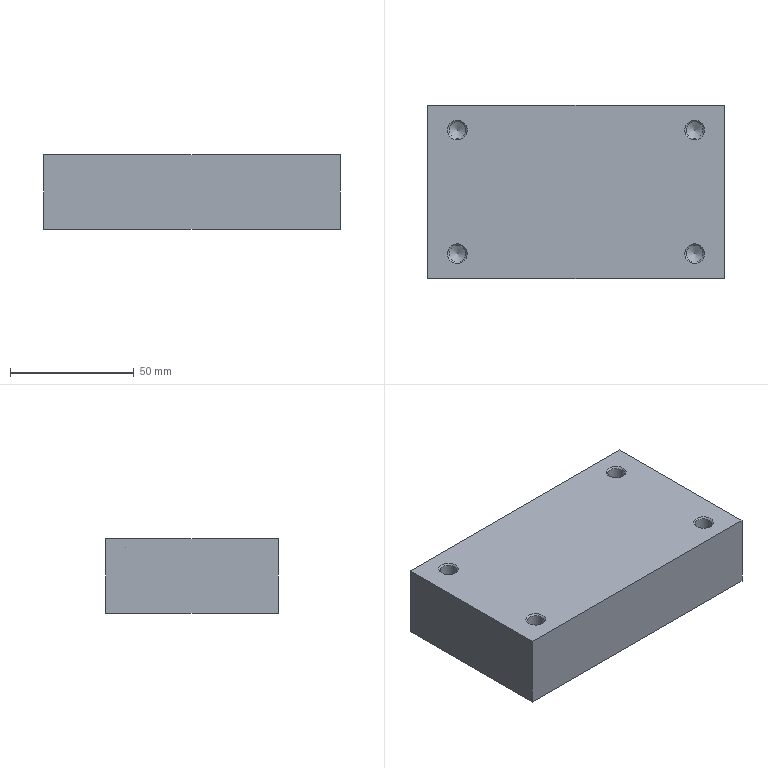Part | STEP file | 冲床-300配套压波_id858_x_t | 1 solid | 18 faces | box 120 x 70 x 30 mm | volume 248979 mm3 | cone 8 | plane 6 | cylinder 4 | commonest cylinder face diameters 6.8 x4
STEP:
#1=CARTESIAN_POINT('',(1760.4,25.,88.));
#2=VERTEX_POINT('',#1);
#3=CARTESIAN_POINT('',(1757.,25.,88.));
#4=DIRECTION('',(0.,0.,1.));
#5=DIRECTION('',(1.,0.,0.));
#6=AXIS2_PLACEMENT_3D('',#3,#4,#5);
#7=CIRCLE('',#6,3.4);
#8=EDGE_CURVE('',#2,#2,#7,.T.);
#9=ORIENTED_EDGE('',*,*,#8,.T.);
#10=EDGE_LOOP('',(#9));
#11=FACE_BOUND('',#10,.T.);
#12=CARTESIAN_POINT('',(1757.,25.,85.957));
#13=VERTEX_POINT('',#12);
#14=VERTEX_LOOP('',#13);
#15=FACE_BOUND('',#14,.T.);
#16=CARTESIAN_POINT('',(1757.,25.,88.));
#17=DIRECTION('',(0.,0.,1.));
#18=DIRECTION('',(-1.,0.,0.));
#19=AXIS2_PLACEMENT_3D('',#16,#17,#18);
#20=CONICAL_SURFACE('',#19,3.4,59.);
#21=ADVANCED_FACE('',(#11,#15),#20,.F.);
#22=CARTESIAN_POINT('',(1753.6,25.,107.4));
#23=VERTEX_POINT('',#22);
#24=CARTESIAN_POINT('',(1757.,25.,107.4));
#25=DIRECTION('',(0.,0.,1.));
#26=DIRECTION('',(-1.,0.,0.));
#27=AXIS2_PLACEMENT_3D('',#24,#25,#26);
#28=CIRCLE('',#27,3.4);
#29=EDGE_CURVE('',#23,#23,#28,.T.);
#30=ORIENTED_EDGE('',*,*,#29,.T.);
#31=EDGE_LOOP('',(#30));
#32=FACE_BOUND('',#31,.T.);
#33=ORIENTED_EDGE('',*,*,#8,.F.);
#34=EDGE_LOOP('',(#33));
#35=FACE_BOUND('',#34,.T.);
#36=CARTESIAN_POINT('',(1757.,25.,108.));
#37=DIRECTION('',(0.,0.,-1.));
#38=DIRECTION('',(1.,0.,0.));
#39=AXIS2_PLACEMENT_3D('',#36,#37,#38);
#40=CYLINDRICAL_SURFACE('',#39,3.4);
#41=ADVANCED_FACE('',(#32,#35),#40,.F.);
#42=ORIENTED_EDGE('',*,*,#29,.F.);
#43=EDGE_LOOP('',(#42));
#44=FACE_BOUND('',#43,.T.);
#45=CARTESIAN_POINT('',(1753.,25.,108.));
#46=VERTEX_POINT('',#45);
#47=CARTESIAN_POINT('',(1757.,25.,108.));
#48=DIRECTION('',(0.,0.,-1.));
#49=DIRECTION('',(-1.,0.,0.));
#50=AXIS2_PLACEMENT_3D('',#47,#48,#49);
#51=CIRCLE('',#50,4.);
#52=EDGE_CURVE('',#46,#46,#51,.T.);
#53=ORIENTED_EDGE('',*,*,#52,.F.);
#54=EDGE_LOOP('',(#53));
#55=FACE_BOUND('',#54,.T.);
#56=CARTESIAN_POINT('',(1757.,25.,108.));
#57=DIRECTION('',(0.,0.,1.));
#58=DIRECTION('',(-1.,0.,0.));
#59=AXIS2_PLACEMENT_3D('',#56,#57,#58);
#60=CONICAL_SURFACE('',#59,4.,45.);
#61=ADVANCED_FACE('',(#44,#55),#60,.F.);
#62=CARTESIAN_POINT('',(1849.6,25.,88.));
#63=VERTEX_POINT('',#62);
#64=CARTESIAN_POINT('',(1853.,25.,88.));
#65=DIRECTION('',(0.,0.,1.));
#66=DIRECTION('',(-1.,0.,0.));
#67=AXIS2_PLACEMENT_3D('',#64,#65,#66);
#68=CIRCLE('',#67,3.4);
#69=EDGE_CURVE('',#63,#63,#68,.T.);
#70=ORIENTED_EDGE('',*,*,#69,.T.);
#71=EDGE_LOOP('',(#70));
#72=FACE_BOUND('',#71,.T.);
#73=CARTESIAN_POINT('',(1853.,25.,85.957));
#74=VERTEX_POINT('',#73);
#75=VERTEX_LOOP('',#74);
#76=FACE_BOUND('',#75,.T.);
#77=CARTESIAN_POINT('',(1853.,25.,88.));
#78=DIRECTION('',(0.,0.,1.));
#79=DIRECTION('',(1.,0.,0.));
#80=AXIS2_PLACEMENT_3D('',#77,#78,#79);
#81=CONICAL_SURFACE('',#80,3.4,59.);
#82=ADVANCED_FACE('',(#72,#76),#81,.F.);
#83=CARTESIAN_POINT('',(1849.6,-25.,88.));
#84=VERTEX_POINT('',#83);
#85=CARTESIAN_POINT('',(1853.,-25.,88.));
#86=DIRECTION('',(0.,0.,1.));
#87=DIRECTION('',(-1.,0.,0.));
#88=AXIS2_PLACEMENT_3D('',#85,#86,#87);
#89=CIRCLE('',#88,3.4);
#90=EDGE_CURVE('',#84,#84,#89,.T.);
#91=ORIENTED_EDGE('',*,*,#90,.T.);
#92=EDGE_LOOP('',(#91));
#93=FACE_BOUND('',#92,.T.);
#94=CARTESIAN_POINT('',(1853.,-25.,85.957));
#95=VERTEX_POINT('',#94);
#96=VERTEX_LOOP('',#95);
#97=FACE_BOUND('',#96,.T.);
#98=CARTESIAN_POINT('',(1853.,-25.,88.));
#99=DIRECTION('',(0.,0.,1.));
#100=DIRECTION('',(1.,0.,0.));
#101=AXIS2_PLACEMENT_3D('',#98,#99,#100);
#102=CONICAL_SURFACE('',#101,3.4,59.);
#103=ADVANCED_FACE('',(#93,#97),#102,.F.);
#104=CARTESIAN_POINT('',(1745.,35.,78.));
#105=VERTEX_POINT('',#104);
#106=CARTESIAN_POINT('',(1745.,-35.,78.));
#107=VERTEX_POINT('',#106);
#108=CARTESIAN_POINT('',(1745.,0.,78.));
#109=DIRECTION('',(0.,-1.,0.));
#110=VECTOR('',#109,1.);
#111=LINE('',#108,#110);
#112=EDGE_CURVE('',#105,#107,#111,.T.);
#113=ORIENTED_EDGE('',*,*,#112,.F.);
#114=CARTESIAN_POINT('',(1865.,35.,78.));
#115=VERTEX_POINT('',#114);
#116=CARTESIAN_POINT('',(60.,35.,78.));
#117=DIRECTION('',(-1.,0.,0.));
#118=VECTOR('',#117,1.);
#119=LINE('',#116,#118);
#120=EDGE_CURVE('',#115,#105,#119,.T.);
#121=ORIENTED_EDGE('',*,*,#120,.F.);
#122=CARTESIAN_POINT('',(1865.,-35.,78.));
#123=VERTEX_POINT('',#122);
#124=CARTESIAN_POINT('',(1865.,0.,78.));
#125=DIRECTION('',(0.,1.,0.));
#126=VECTOR('',#125,1.);
#127=LINE('',#124,#126);
#128=EDGE_CURVE('',#123,#115,#127,.T.);
#129=ORIENTED_EDGE('',*,*,#128,.F.);
#130=CARTESIAN_POINT('',(60.,-35.,78.));
#131=DIRECTION('',(1.,0.,0.));
#132=VECTOR('',#131,1.);
#133=LINE('',#130,#132);
#134=EDGE_CURVE('',#107,#123,#133,.T.);
#135=ORIENTED_EDGE('',*,*,#134,.F.);
#136=EDGE_LOOP('',(#113,#121,#129,#135));
#137=FACE_OUTER_BOUND('',#136,.T.);
#138=CARTESIAN_POINT('',(60.,0.,78.));
#139=DIRECTION('',(0.,0.,1.));
#140=DIRECTION('',(1.,0.,0.));
#141=AXIS2_PLACEMENT_3D('',#138,#139,#140);
#142=PLANE('',#141);
#143=ADVANCED_FACE('',(#137),#142,.F.);
#144=CARTESIAN_POINT('',(1856.4,25.,107.4));
#145=VERTEX_POINT('',#144);
#146=CARTESIAN_POINT('',(1853.,25.,107.4));
#147=DIRECTION('',(0.,0.,1.));
#148=DIRECTION('',(1.,0.,0.));
#149=AXIS2_PLACEMENT_3D('',#146,#147,#148);
#150=CIRCLE('',#149,3.4);
#151=EDGE_CURVE('',#145,#145,#150,.T.);
#152=ORIENTED_EDGE('',*,*,#151,.T.);
#153=EDGE_LOOP('',(#152));
#154=FACE_BOUND('',#153,.T.);
#155=ORIENTED_EDGE('',*,*,#69,.F.);
#156=EDGE_LOOP('',(#155));
#157=FACE_BOUND('',#156,.T.);
#158=CARTESIAN_POINT('',(1853.,25.,108.));
#159=DIRECTION('',(0.,0.,-1.));
#160=DIRECTION('',(-1.,0.,0.));
#161=AXIS2_PLACEMENT_3D('',#158,#159,#160);
#162=CYLINDRICAL_SURFACE('',#161,3.4);
#163=ADVANCED_FACE('',(#154,#157),#162,.F.);
#164=CARTESIAN_POINT('',(1856.4,-25.,107.4));
#165=VERTEX_POINT('',#164);
#166=CARTESIAN_POINT('',(1853.,-25.,107.4));
#167=DIRECTION('',(0.,0.,1.));
#168=DIRECTION('',(1.,0.,0.));
#169=AXIS2_PLACEMENT_3D('',#166,#167,#168);
#170=CIRCLE('',#169,3.4);
#171=EDGE_CURVE('',#165,#165,#170,.T.);
#172=ORIENTED_EDGE('',*,*,#171,.T.);
#173=EDGE_LOOP('',(#172));
#174=FACE_BOUND('',#173,.T.);
#175=ORIENTED_EDGE('',*,*,#90,.F.);
#176=EDGE_LOOP('',(#175));
#177=FACE_BOUND('',#176,.T.);
#178=CARTESIAN_POINT('',(1853.,-25.,108.));
#179=DIRECTION('',(0.,0.,-1.));
#180=DIRECTION('',(-1.,0.,0.));
#181=AXIS2_PLACEMENT_3D('',#178,#179,#180);
#182=CYLINDRICAL_SURFACE('',#181,3.4);
#183=ADVANCED_FACE('',(#174,#177),#182,.F.);
#184=CARTESIAN_POINT('',(1865.,35.,108.));
#185=VERTEX_POINT('',#184);
#186=CARTESIAN_POINT('',(1745.,35.,108.));
#187=VERTEX_POINT('',#186);
#188=CARTESIAN_POINT('',(60.,35.,108.));
#189=DIRECTION('',(-1.,0.,0.));
#190=VECTOR('',#189,1.);
#191=LINE('',#188,#190);
#192=EDGE_CURVE('',#185,#187,#191,.T.);
#193=ORIENTED_EDGE('',*,*,#192,.F.);
#194=CARTESIAN_POINT('',(1865.,35.,88.));
#195=DIRECTION('',(0.,0.,1.));
#196=VECTOR('',#195,1.);
#197=LINE('',#194,#196);
#198=EDGE_CURVE('',#115,#185,#197,.T.);
#199=ORIENTED_EDGE('',*,*,#198,.F.);
#200=ORIENTED_EDGE('',*,*,#120,.T.);
#201=CARTESIAN_POINT('',(1745.,35.,88.));
#202=DIRECTION('',(0.,0.,1.));
#203=VECTOR('',#202,1.);
#204=LINE('',#201,#203);
#205=EDGE_CURVE('',#105,#187,#204,.T.);
#206=ORIENTED_EDGE('',*,*,#205,.T.);
#207=EDGE_LOOP('',(#193,#199,#200,#206));
#208=FACE_OUTER_BOUND('',#207,.T.);
#209=CARTESIAN_POINT('',(1880.,35.,88.));
#210=DIRECTION('',(0.,1.,0.));
#211=DIRECTION('',(0.,0.,1.));
#212=AXIS2_PLACEMENT_3D('',#209,#210,#211);
#213=PLANE('',#212);
#214=ADVANCED_FACE('',(#208),#213,.T.);
#215=CARTESIAN_POINT('',(1865.,-35.,108.));
#216=VERTEX_POINT('',#215);
#217=CARTESIAN_POINT('',(1865.,0.,108.));
#218=DIRECTION('',(0.,1.,0.));
#219=VECTOR('',#218,1.);
#220=LINE('',#217,#219);
#221=EDGE_CURVE('',#216,#185,#220,.T.);
#222=ORIENTED_EDGE('',*,*,#221,.F.);
#223=CARTESIAN_POINT('',(1865.,-35.,88.));
#224=DIRECTION('',(0.,0.,1.));
#225=VECTOR('',#224,1.);
#226=LINE('',#223,#225);
#227=EDGE_CURVE('',#123,#216,#226,.T.);
#228=ORIENTED_EDGE('',*,*,#227,.F.);
#229=ORIENTED_EDGE('',*,*,#128,.T.);
#230=ORIENTED_EDGE('',*,*,#198,.T.);
#231=EDGE_LOOP('',(#222,#228,#229,#230));
#232=FACE_OUTER_BOUND('',#231,.T.);
#233=CARTESIAN_POINT('',(1865.,-60.,88.));
#234=DIRECTION('',(1.,0.,0.));
#235=DIRECTION('',(0.,0.,-1.));
#236=AXIS2_PLACEMENT_3D('',#233,#234,#235);
#237=PLANE('',#236);
#238=ADVANCED_FACE('',(#232),#237,.T.);
#239=CARTESIAN_POINT('',(1745.,-35.,108.));
#240=VERTEX_POINT('',#239);
#241=CARTESIAN_POINT('',(60.,-35.,108.));
#242=DIRECTION('',(1.,0.,0.));
#243=VECTOR('',#242,1.);
#244=LINE('',#241,#243);
#245=EDGE_CURVE('',#240,#216,#244,.T.);
#246=ORIENTED_EDGE('',*,*,#245,.F.);
#247=CARTESIAN_POINT('',(1745.,-35.,88.));
#248=DIRECTION('',(0.,0.,1.));
#249=VECTOR('',#248,1.);
#250=LINE('',#247,#249);
#251=EDGE_CURVE('',#107,#240,#250,.T.);
#252=ORIENTED_EDGE('',*,*,#251,.F.);
#253=ORIENTED_EDGE('',*,*,#134,.T.);
#254=ORIENTED_EDGE('',*,*,#227,.T.);
#255=EDGE_LOOP('',(#246,#252,#253,#254));
#256=FACE_OUTER_BOUND('',#255,.T.);
#257=CARTESIAN_POINT('',(1730.,-35.,88.));
#258=DIRECTION('',(0.,-1.,0.));
#259=DIRECTION('',(0.,0.,-1.));
#260=AXIS2_PLACEMENT_3D('',#257,#258,#259);
#261=PLANE('',#260);
#262=ADVANCED_FACE('',(#256),#261,.T.);
#263=CARTESIAN_POINT('',(1745.,0.,108.));
#264=DIRECTION('',(0.,-1.,0.));
#265=VECTOR('',#264,1.);
#266=LINE('',#263,#265);
#267=EDGE_CURVE('',#187,#240,#266,.T.);
#268=ORIENTED_EDGE('',*,*,#267,.F.);
#269=ORIENTED_EDGE('',*,*,#205,.F.);
#270=ORIENTED_EDGE('',*,*,#112,.T.);
#271=ORIENTED_EDGE('',*,*,#251,.T.);
#272=EDGE_LOOP('',(#268,#269,#270,#271));
#273=FACE_OUTER_BOUND('',#272,.T.);
#274=CARTESIAN_POINT('',(1745.,60.,88.));
#275=DIRECTION('',(-1.,0.,0.));
#276=DIRECTION('',(0.,0.,1.));
#277=AXIS2_PLACEMENT_3D('',#274,#275,#276);
#278=PLANE('',#277);
#279=ADVANCED_FACE('',(#273),#278,.T.);
#280=ORIENTED_EDGE('',*,*,#151,.F.);
#281=EDGE_LOOP('',(#280));
#282=FACE_BOUND('',#281,.T.);
#283=CARTESIAN_POINT('',(1857.,25.,108.));
#284=VERTEX_POINT('',#283);
#285=CARTESIAN_POINT('',(1853.,25.,108.));
#286=DIRECTION('',(0.,0.,-1.));
#287=DIRECTION('',(1.,0.,0.));
#288=AXIS2_PLACEMENT_3D('',#285,#286,#287);
#289=CIRCLE('',#288,4.);
#290=EDGE_CURVE('',#284,#284,#289,.T.);
#291=ORIENTED_EDGE('',*,*,#290,.F.);
#292=EDGE_LOOP('',(#291));
#293=FACE_BOUND('',#292,.T.);
#294=CARTESIAN_POINT('',(1853.,25.,108.));
#295=DIRECTION('',(0.,0.,1.));
#296=DIRECTION('',(1.,0.,0.));
#297=AXIS2_PLACEMENT_3D('',#294,#295,#296);
#298=CONICAL_SURFACE('',#297,4.,45.);
#299=ADVANCED_FACE('',(#282,#293),#298,.F.);
#300=ORIENTED_EDGE('',*,*,#171,.F.);
#301=EDGE_LOOP('',(#300));
#302=FACE_BOUND('',#301,.T.);
#303=CARTESIAN_POINT('',(1857.,-25.,108.));
#304=VERTEX_POINT('',#303);
#305=CARTESIAN_POINT('',(1853.,-25.,108.));
#306=DIRECTION('',(0.,0.,-1.));
#307=DIRECTION('',(1.,0.,0.));
#308=AXIS2_PLACEMENT_3D('',#305,#306,#307);
#309=CIRCLE('',#308,4.);
#310=EDGE_CURVE('',#304,#304,#309,.T.);
#311=ORIENTED_EDGE('',*,*,#310,.F.);
#312=EDGE_LOOP('',(#311));
#313=FACE_BOUND('',#312,.T.);
#314=CARTESIAN_POINT('',(1853.,-25.,108.));
#315=DIRECTION('',(0.,0.,1.));
#316=DIRECTION('',(1.,0.,0.));
#317=AXIS2_PLACEMENT_3D('',#314,#315,#316);
#318=CONICAL_SURFACE('',#317,4.,45.);
#319=ADVANCED_FACE('',(#302,#313),#318,.F.);
#320=CARTESIAN_POINT('',(1753.,-25.,108.));
#321=VERTEX_POINT('',#320);
#322=CARTESIAN_POINT('',(1757.,-25.,108.));
#323=DIRECTION('',(0.,0.,-1.));
#324=DIRECTION('',(-1.,0.,0.));
#325=AXIS2_PLACEMENT_3D('',#322,#323,#324);
#326=CIRCLE('',#325,4.);
#327=EDGE_CURVE('',#321,#321,#326,.T.);
#328=ORIENTED_EDGE('',*,*,#327,.T.);
#329=EDGE_LOOP('',(#328));
#330=FACE_BOUND('',#329,.T.);
#331=ORIENTED_EDGE('',*,*,#52,.T.);
#332=EDGE_LOOP('',(#331));
#333=FACE_BOUND('',#332,.T.);
#334=ORIENTED_EDGE('',*,*,#310,.T.);
#335=EDGE_LOOP('',(#334));
#336=FACE_BOUND('',#335,.T.);
#337=ORIENTED_EDGE('',*,*,#290,.T.);
#338=EDGE_LOOP('',(#337));
#339=FACE_BOUND('',#338,.T.);
#340=ORIENTED_EDGE('',*,*,#267,.T.);
#341=ORIENTED_EDGE('',*,*,#245,.T.);
#342=ORIENTED_EDGE('',*,*,#221,.T.);
#343=ORIENTED_EDGE('',*,*,#192,.T.);
#344=EDGE_LOOP('',(#340,#341,#342,#343));
#345=FACE_BOUND('',#344,.T.);
#346=CARTESIAN_POINT('',(60.,0.,108.));
#347=DIRECTION('',(0.,0.,1.));
#348=DIRECTION('',(1.,0.,0.));
#349=AXIS2_PLACEMENT_3D('',#346,#347,#348);
#350=PLANE('',#349);
#351=ADVANCED_FACE('',(#330,#333,#336,#339,#345),#350,.T.);
#352=CARTESIAN_POINT('',(1760.4,-25.,88.));
#353=VERTEX_POINT('',#352);
#354=CARTESIAN_POINT('',(1757.,-25.,88.));
#355=DIRECTION('',(0.,0.,1.));
#356=DIRECTION('',(1.,0.,0.));
#357=AXIS2_PLACEMENT_3D('',#354,#355,#356);
#358=CIRCLE('',#357,3.4);
#359=EDGE_CURVE('',#353,#353,#358,.T.);
#360=ORIENTED_EDGE('',*,*,#359,.T.);
#361=EDGE_LOOP('',(#360));
#362=FACE_BOUND('',#361,.T.);
#363=CARTESIAN_POINT('',(1757.,-25.,85.957));
#364=VERTEX_POINT('',#363);
#365=VERTEX_LOOP('',#364);
#366=FACE_BOUND('',#365,.T.);
#367=CARTESIAN_POINT('',(1757.,-25.,88.));
#368=DIRECTION('',(0.,0.,1.));
#369=DIRECTION('',(-1.,0.,0.));
#370=AXIS2_PLACEMENT_3D('',#367,#368,#369);
#371=CONICAL_SURFACE('',#370,3.4,59.);
#372=ADVANCED_FACE('',(#362,#366),#371,.F.);
#373=CARTESIAN_POINT('',(1753.6,-25.,107.4));
#374=VERTEX_POINT('',#373);
#375=CARTESIAN_POINT('',(1757.,-25.,107.4));
#376=DIRECTION('',(0.,0.,1.));
#377=DIRECTION('',(-1.,0.,0.));
#378=AXIS2_PLACEMENT_3D('',#375,#376,#377);
#379=CIRCLE('',#378,3.4);
#380=EDGE_CURVE('',#374,#374,#379,.T.);
#381=ORIENTED_EDGE('',*,*,#380,.T.);
#382=EDGE_LOOP('',(#381));
#383=FACE_BOUND('',#382,.T.);
#384=ORIENTED_EDGE('',*,*,#359,.F.);
#385=EDGE_LOOP('',(#384));
#386=FACE_BOUND('',#385,.T.);
#387=CARTESIAN_POINT('',(1757.,-25.,108.));
#388=DIRECTION('',(0.,0.,-1.));
#389=DIRECTION('',(1.,0.,0.));
#390=AXIS2_PLACEMENT_3D('',#387,#388,#389);
#391=CYLINDRICAL_SURFACE('',#390,3.4);
#392=ADVANCED_FACE('',(#383,#386),#391,.F.);
#393=ORIENTED_EDGE('',*,*,#380,.F.);
#394=EDGE_LOOP('',(#393));
#395=FACE_BOUND('',#394,.T.);
#396=ORIENTED_EDGE('',*,*,#327,.F.);
#397=EDGE_LOOP('',(#396));
#398=FACE_BOUND('',#397,.T.);
#399=CARTESIAN_POINT('',(1757.,-25.,108.));
#400=DIRECTION('',(0.,0.,1.));
#401=DIRECTION('',(-1.,0.,0.));
#402=AXIS2_PLACEMENT_3D('',#399,#400,#401);
#403=CONICAL_SURFACE('',#402,4.,45.);
#404=ADVANCED_FACE('',(#395,#398),#403,.F.);
#405=CLOSED_SHELL('',(#21,#41,#61,#82,#103,#143,#163,#183,#214,#238,#262,#279,#299,#319,#351,#372,#392,#404));
#406=MANIFOLD_SOLID_BREP('',#405);
#407=(LENGTH_UNIT()NAMED_UNIT(*)SI_UNIT(.MILLI.,.METRE.));
#408=UNCERTAINTY_MEASURE_WITH_UNIT(LENGTH_MEASURE(0.00002),#407,'','');
#409=(NAMED_UNIT(*)PLANE_ANGLE_UNIT()SI_UNIT($,.RADIAN.));
#410=PLANE_ANGLE_MEASURE_WITH_UNIT(PLANE_ANGLE_MEASURE(0.01745),#409);
#411=DIMENSIONAL_EXPONENTS(0.,0.,0.,0.,0.,0.,0.);
#412=(CONVERSION_BASED_UNIT('DEGREE',#410)NAMED_UNIT(#411)PLANE_ANGLE_UNIT());
#413=(NAMED_UNIT(*)SI_UNIT($,.STERADIAN.)SOLID_ANGLE_UNIT());
#414=(GEOMETRIC_REPRESENTATION_CONTEXT(3)GLOBAL_UNCERTAINTY_ASSIGNED_CONTEXT((#408))GLOBAL_UNIT_ASSIGNED_CONTEXT((#407,#412,#413))REPRESENTATION_CONTEXT('',''));
#415=ADVANCED_BREP_SHAPE_REPRESENTATION('',(#406),#414);